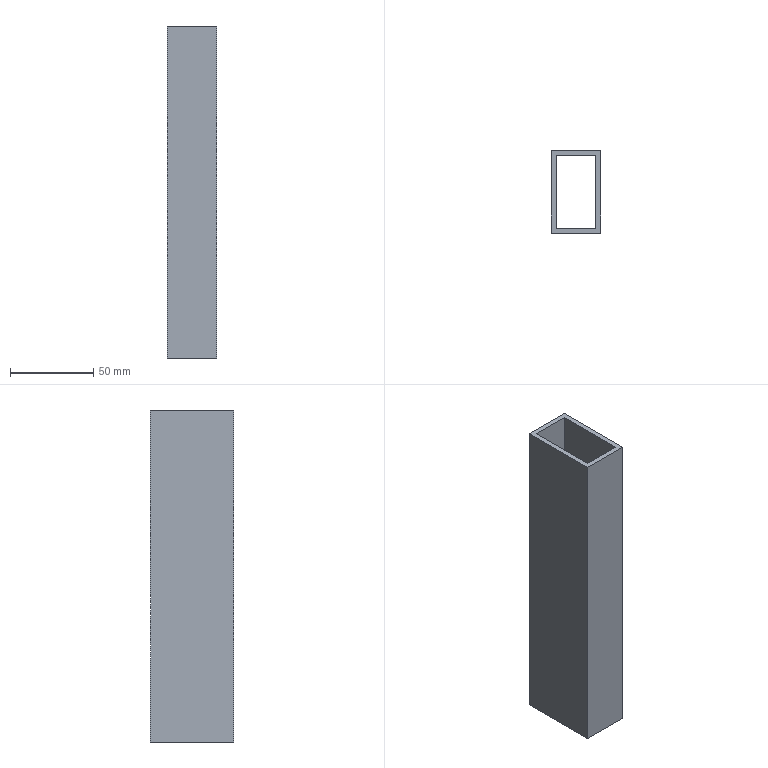Part | SolidWorks | features Extrusion 1 | 1 solid | 10 faces | box 30 x 50 x 200 mm | volume 88800 mm3 | plane 10
STEP:
#1=CARTESIAN_POINT('',(-15.,25.,100.));
#2=VERTEX_POINT('',#1);
#3=CARTESIAN_POINT('',(-15.,-25.,100.));
#4=VERTEX_POINT('',#3);
#5=CARTESIAN_POINT('',(-15.,25.,100.));
#6=DIRECTION('',(0.,-1.,0.));
#7=VECTOR('',#6,1000.);
#8=LINE('',#5,#7);
#9=EDGE_CURVE('',#2,#4,#8,.T.);
#10=ORIENTED_EDGE('',*,*,#9,.F.);
#11=CARTESIAN_POINT('',(-15.,25.,-100.));
#12=VERTEX_POINT('',#11);
#13=CARTESIAN_POINT('',(-15.,25.,-100.));
#14=DIRECTION('',(0.,0.,1.));
#15=VECTOR('',#14,1000.);
#16=LINE('',#13,#15);
#17=EDGE_CURVE('',#12,#2,#16,.T.);
#18=ORIENTED_EDGE('',*,*,#17,.F.);
#19=CARTESIAN_POINT('',(-15.,-25.,-100.));
#20=VERTEX_POINT('',#19);
#21=CARTESIAN_POINT('',(-15.,25.,-100.));
#22=DIRECTION('',(0.,-1.,0.));
#23=VECTOR('',#22,1000.);
#24=LINE('',#21,#23);
#25=EDGE_CURVE('',#12,#20,#24,.T.);
#26=ORIENTED_EDGE('',*,*,#25,.T.);
#27=CARTESIAN_POINT('',(-15.,-25.,-100.));
#28=DIRECTION('',(0.,0.,1.));
#29=VECTOR('',#28,1000.);
#30=LINE('',#27,#29);
#31=EDGE_CURVE('',#20,#4,#30,.T.);
#32=ORIENTED_EDGE('',*,*,#31,.T.);
#33=EDGE_LOOP('',(#10,#18,#26,#32));
#34=FACE_OUTER_BOUND('',#33,.T.);
#35=CARTESIAN_POINT('',(-15.,25.,-100.));
#36=DIRECTION('',(-1.,0.,0.));
#37=DIRECTION('',(0.,0.,1.));
#38=AXIS2_PLACEMENT_3D('',#35,#36,#37);
#39=PLANE('',#38);
#40=ADVANCED_FACE('',(#34),#39,.T.);
#41=CARTESIAN_POINT('',(15.,25.,100.));
#42=VERTEX_POINT('',#41);
#43=CARTESIAN_POINT('',(15.,25.,100.));
#44=DIRECTION('',(-1.,0.,0.));
#45=VECTOR('',#44,1000.);
#46=LINE('',#43,#45);
#47=EDGE_CURVE('',#42,#2,#46,.T.);
#48=ORIENTED_EDGE('',*,*,#47,.F.);
#49=CARTESIAN_POINT('',(15.,25.,-100.));
#50=VERTEX_POINT('',#49);
#51=CARTESIAN_POINT('',(15.,25.,-100.));
#52=DIRECTION('',(0.,0.,1.));
#53=VECTOR('',#52,1000.);
#54=LINE('',#51,#53);
#55=EDGE_CURVE('',#50,#42,#54,.T.);
#56=ORIENTED_EDGE('',*,*,#55,.F.);
#57=CARTESIAN_POINT('',(15.,25.,-100.));
#58=DIRECTION('',(-1.,0.,0.));
#59=VECTOR('',#58,1000.);
#60=LINE('',#57,#59);
#61=EDGE_CURVE('',#50,#12,#60,.T.);
#62=ORIENTED_EDGE('',*,*,#61,.T.);
#63=ORIENTED_EDGE('',*,*,#17,.T.);
#64=EDGE_LOOP('',(#48,#56,#62,#63));
#65=FACE_OUTER_BOUND('',#64,.T.);
#66=CARTESIAN_POINT('',(15.,25.,-100.));
#67=DIRECTION('',(0.,1.,0.));
#68=DIRECTION('',(0.,0.,1.));
#69=AXIS2_PLACEMENT_3D('',#66,#67,#68);
#70=PLANE('',#69);
#71=ADVANCED_FACE('',(#65),#70,.T.);
#72=CARTESIAN_POINT('',(15.,-25.,100.));
#73=VERTEX_POINT('',#72);
#74=CARTESIAN_POINT('',(15.,-25.,100.));
#75=DIRECTION('',(0.,1.,0.));
#76=VECTOR('',#75,1000.);
#77=LINE('',#74,#76);
#78=EDGE_CURVE('',#73,#42,#77,.T.);
#79=ORIENTED_EDGE('',*,*,#78,.F.);
#80=CARTESIAN_POINT('',(15.,-25.,-100.));
#81=VERTEX_POINT('',#80);
#82=CARTESIAN_POINT('',(15.,-25.,-100.));
#83=DIRECTION('',(0.,0.,1.));
#84=VECTOR('',#83,1000.);
#85=LINE('',#82,#84);
#86=EDGE_CURVE('',#81,#73,#85,.T.);
#87=ORIENTED_EDGE('',*,*,#86,.F.);
#88=CARTESIAN_POINT('',(15.,-25.,-100.));
#89=DIRECTION('',(0.,1.,0.));
#90=VECTOR('',#89,1000.);
#91=LINE('',#88,#90);
#92=EDGE_CURVE('',#81,#50,#91,.T.);
#93=ORIENTED_EDGE('',*,*,#92,.T.);
#94=ORIENTED_EDGE('',*,*,#55,.T.);
#95=EDGE_LOOP('',(#79,#87,#93,#94));
#96=FACE_OUTER_BOUND('',#95,.T.);
#97=CARTESIAN_POINT('',(15.,-25.,-100.));
#98=DIRECTION('',(1.,0.,0.));
#99=DIRECTION('',(0.,0.,-1.));
#100=AXIS2_PLACEMENT_3D('',#97,#98,#99);
#101=PLANE('',#100);
#102=ADVANCED_FACE('',(#96),#101,.T.);
#103=CARTESIAN_POINT('',(-15.,-25.,100.));
#104=DIRECTION('',(1.,0.,0.));
#105=VECTOR('',#104,1000.);
#106=LINE('',#103,#105);
#107=EDGE_CURVE('',#4,#73,#106,.T.);
#108=ORIENTED_EDGE('',*,*,#107,.F.);
#109=ORIENTED_EDGE('',*,*,#31,.F.);
#110=CARTESIAN_POINT('',(-15.,-25.,-100.));
#111=DIRECTION('',(1.,0.,0.));
#112=VECTOR('',#111,1000.);
#113=LINE('',#110,#112);
#114=EDGE_CURVE('',#20,#81,#113,.T.);
#115=ORIENTED_EDGE('',*,*,#114,.T.);
#116=ORIENTED_EDGE('',*,*,#86,.T.);
#117=EDGE_LOOP('',(#108,#109,#115,#116));
#118=FACE_OUTER_BOUND('',#117,.T.);
#119=CARTESIAN_POINT('',(-15.,-25.,-100.));
#120=DIRECTION('',(0.,-1.,0.));
#121=DIRECTION('',(0.,0.,-1.));
#122=AXIS2_PLACEMENT_3D('',#119,#120,#121);
#123=PLANE('',#122);
#124=ADVANCED_FACE('',(#118),#123,.T.);
#125=CARTESIAN_POINT('',(12.,22.,-100.));
#126=VERTEX_POINT('',#125);
#127=CARTESIAN_POINT('',(-12.,22.,-100.));
#128=VERTEX_POINT('',#127);
#129=CARTESIAN_POINT('',(12.,22.,-100.));
#130=DIRECTION('',(-1.,0.,0.));
#131=VECTOR('',#130,1000.);
#132=LINE('',#129,#131);
#133=EDGE_CURVE('',#126,#128,#132,.T.);
#134=ORIENTED_EDGE('',*,*,#133,.T.);
#135=CARTESIAN_POINT('',(-12.,-22.,-100.));
#136=VERTEX_POINT('',#135);
#137=CARTESIAN_POINT('',(-12.,22.,-100.));
#138=DIRECTION('',(0.,-1.,0.));
#139=VECTOR('',#138,1000.);
#140=LINE('',#137,#139);
#141=EDGE_CURVE('',#128,#136,#140,.T.);
#142=ORIENTED_EDGE('',*,*,#141,.T.);
#143=CARTESIAN_POINT('',(12.,-22.,-100.));
#144=VERTEX_POINT('',#143);
#145=CARTESIAN_POINT('',(-12.,-22.,-100.));
#146=DIRECTION('',(1.,0.,0.));
#147=VECTOR('',#146,1000.);
#148=LINE('',#145,#147);
#149=EDGE_CURVE('',#136,#144,#148,.T.);
#150=ORIENTED_EDGE('',*,*,#149,.T.);
#151=CARTESIAN_POINT('',(12.,-22.,-100.));
#152=DIRECTION('',(0.,1.,0.));
#153=VECTOR('',#152,1000.);
#154=LINE('',#151,#153);
#155=EDGE_CURVE('',#144,#126,#154,.T.);
#156=ORIENTED_EDGE('',*,*,#155,.T.);
#157=EDGE_LOOP('',(#134,#142,#150,#156));
#158=FACE_BOUND('',#157,.T.);
#159=ORIENTED_EDGE('',*,*,#25,.F.);
#160=ORIENTED_EDGE('',*,*,#61,.F.);
#161=ORIENTED_EDGE('',*,*,#92,.F.);
#162=ORIENTED_EDGE('',*,*,#114,.F.);
#163=EDGE_LOOP('',(#159,#160,#161,#162));
#164=FACE_OUTER_BOUND('',#163,.T.);
#165=CARTESIAN_POINT('',(0.,0.,-100.));
#166=DIRECTION('',(0.,0.,1.));
#167=DIRECTION('',(1.,0.,0.));
#168=AXIS2_PLACEMENT_3D('',#165,#166,#167);
#169=PLANE('',#168);
#170=ADVANCED_FACE('',(#158,#164),#169,.F.);
#171=CARTESIAN_POINT('',(-12.,22.,100.));
#172=VERTEX_POINT('',#171);
#173=CARTESIAN_POINT('',(-12.,-22.,100.));
#174=VERTEX_POINT('',#173);
#175=CARTESIAN_POINT('',(-12.,22.,100.));
#176=DIRECTION('',(0.,-1.,0.));
#177=VECTOR('',#176,1000.);
#178=LINE('',#175,#177);
#179=EDGE_CURVE('',#172,#174,#178,.T.);
#180=ORIENTED_EDGE('',*,*,#179,.F.);
#181=CARTESIAN_POINT('',(12.,22.,100.));
#182=VERTEX_POINT('',#181);
#183=CARTESIAN_POINT('',(12.,22.,100.));
#184=DIRECTION('',(-1.,0.,0.));
#185=VECTOR('',#184,1000.);
#186=LINE('',#183,#185);
#187=EDGE_CURVE('',#182,#172,#186,.T.);
#188=ORIENTED_EDGE('',*,*,#187,.F.);
#189=CARTESIAN_POINT('',(12.,-22.,100.));
#190=VERTEX_POINT('',#189);
#191=CARTESIAN_POINT('',(12.,-22.,100.));
#192=DIRECTION('',(0.,1.,0.));
#193=VECTOR('',#192,1000.);
#194=LINE('',#191,#193);
#195=EDGE_CURVE('',#190,#182,#194,.T.);
#196=ORIENTED_EDGE('',*,*,#195,.F.);
#197=CARTESIAN_POINT('',(-12.,-22.,100.));
#198=DIRECTION('',(1.,0.,0.));
#199=VECTOR('',#198,1000.);
#200=LINE('',#197,#199);
#201=EDGE_CURVE('',#174,#190,#200,.T.);
#202=ORIENTED_EDGE('',*,*,#201,.F.);
#203=EDGE_LOOP('',(#180,#188,#196,#202));
#204=FACE_BOUND('',#203,.T.);
#205=ORIENTED_EDGE('',*,*,#9,.T.);
#206=ORIENTED_EDGE('',*,*,#107,.T.);
#207=ORIENTED_EDGE('',*,*,#78,.T.);
#208=ORIENTED_EDGE('',*,*,#47,.T.);
#209=EDGE_LOOP('',(#205,#206,#207,#208));
#210=FACE_OUTER_BOUND('',#209,.T.);
#211=CARTESIAN_POINT('',(0.,0.,100.));
#212=DIRECTION('',(0.,0.,1.));
#213=DIRECTION('',(1.,0.,0.));
#214=AXIS2_PLACEMENT_3D('',#211,#212,#213);
#215=PLANE('',#214);
#216=ADVANCED_FACE('',(#204,#210),#215,.T.);
#217=ORIENTED_EDGE('',*,*,#179,.T.);
#218=CARTESIAN_POINT('',(-12.,-22.,-100.));
#219=DIRECTION('',(0.,0.,1.));
#220=VECTOR('',#219,1000.);
#221=LINE('',#218,#220);
#222=EDGE_CURVE('',#136,#174,#221,.T.);
#223=ORIENTED_EDGE('',*,*,#222,.F.);
#224=ORIENTED_EDGE('',*,*,#141,.F.);
#225=CARTESIAN_POINT('',(-12.,22.,-100.));
#226=DIRECTION('',(0.,0.,1.));
#227=VECTOR('',#226,1000.);
#228=LINE('',#225,#227);
#229=EDGE_CURVE('',#128,#172,#228,.T.);
#230=ORIENTED_EDGE('',*,*,#229,.T.);
#231=EDGE_LOOP('',(#217,#223,#224,#230));
#232=FACE_OUTER_BOUND('',#231,.T.);
#233=CARTESIAN_POINT('',(-12.,22.,-100.));
#234=DIRECTION('',(-1.,0.,0.));
#235=DIRECTION('',(0.,0.,1.));
#236=AXIS2_PLACEMENT_3D('',#233,#234,#235);
#237=PLANE('',#236);
#238=ADVANCED_FACE('',(#232),#237,.F.);
#239=ORIENTED_EDGE('',*,*,#187,.T.);
#240=ORIENTED_EDGE('',*,*,#229,.F.);
#241=ORIENTED_EDGE('',*,*,#133,.F.);
#242=CARTESIAN_POINT('',(12.,22.,-100.));
#243=DIRECTION('',(0.,0.,1.));
#244=VECTOR('',#243,1000.);
#245=LINE('',#242,#244);
#246=EDGE_CURVE('',#126,#182,#245,.T.);
#247=ORIENTED_EDGE('',*,*,#246,.T.);
#248=EDGE_LOOP('',(#239,#240,#241,#247));
#249=FACE_OUTER_BOUND('',#248,.T.);
#250=CARTESIAN_POINT('',(12.,22.,-100.));
#251=DIRECTION('',(0.,1.,0.));
#252=DIRECTION('',(0.,0.,1.));
#253=AXIS2_PLACEMENT_3D('',#250,#251,#252);
#254=PLANE('',#253);
#255=ADVANCED_FACE('',(#249),#254,.F.);
#256=ORIENTED_EDGE('',*,*,#195,.T.);
#257=ORIENTED_EDGE('',*,*,#246,.F.);
#258=ORIENTED_EDGE('',*,*,#155,.F.);
#259=CARTESIAN_POINT('',(12.,-22.,-100.));
#260=DIRECTION('',(0.,0.,1.));
#261=VECTOR('',#260,1000.);
#262=LINE('',#259,#261);
#263=EDGE_CURVE('',#144,#190,#262,.T.);
#264=ORIENTED_EDGE('',*,*,#263,.T.);
#265=EDGE_LOOP('',(#256,#257,#258,#264));
#266=FACE_OUTER_BOUND('',#265,.T.);
#267=CARTESIAN_POINT('',(12.,-22.,-100.));
#268=DIRECTION('',(1.,0.,0.));
#269=DIRECTION('',(0.,0.,-1.));
#270=AXIS2_PLACEMENT_3D('',#267,#268,#269);
#271=PLANE('',#270);
#272=ADVANCED_FACE('',(#266),#271,.F.);
#273=ORIENTED_EDGE('',*,*,#201,.T.);
#274=ORIENTED_EDGE('',*,*,#263,.F.);
#275=ORIENTED_EDGE('',*,*,#149,.F.);
#276=ORIENTED_EDGE('',*,*,#222,.T.);
#277=EDGE_LOOP('',(#273,#274,#275,#276));
#278=FACE_OUTER_BOUND('',#277,.T.);
#279=CARTESIAN_POINT('',(-12.,-22.,-100.));
#280=DIRECTION('',(0.,-1.,0.));
#281=DIRECTION('',(0.,0.,-1.));
#282=AXIS2_PLACEMENT_3D('',#279,#280,#281);
#283=PLANE('',#282);
#284=ADVANCED_FACE('',(#278),#283,.F.);
#285=CLOSED_SHELL('',(#40,#71,#102,#124,#170,#216,#238,#255,#272,#284));
#286=MANIFOLD_SOLID_BREP('',#285);
#287=CARTESIAN_POINT('',(0.,0.,0.));
#288=DIRECTION('',(0.,0.,1.));
#289=DIRECTION('',(1.,0.,0.));
#290=AXIS2_PLACEMENT_3D('',#287,#288,#289);
#291=(LENGTH_UNIT()NAMED_UNIT(*)SI_UNIT(.MILLI.,.METRE.));
#292=UNCERTAINTY_MEASURE_WITH_UNIT(LENGTH_MEASURE(0.00001),#291,'','');
#293=(NAMED_UNIT(*)PLANE_ANGLE_UNIT()SI_UNIT($,.RADIAN.));
#294=(NAMED_UNIT(*)SI_UNIT($,.STERADIAN.)SOLID_ANGLE_UNIT());
#295=(GEOMETRIC_REPRESENTATION_CONTEXT(3)GLOBAL_UNCERTAINTY_ASSIGNED_CONTEXT((#292))GLOBAL_UNIT_ASSIGNED_CONTEXT((#291,#293,#294))REPRESENTATION_CONTEXT('',''));
#296=ADVANCED_BREP_SHAPE_REPRESENTATION('',(#286,#290),#295);